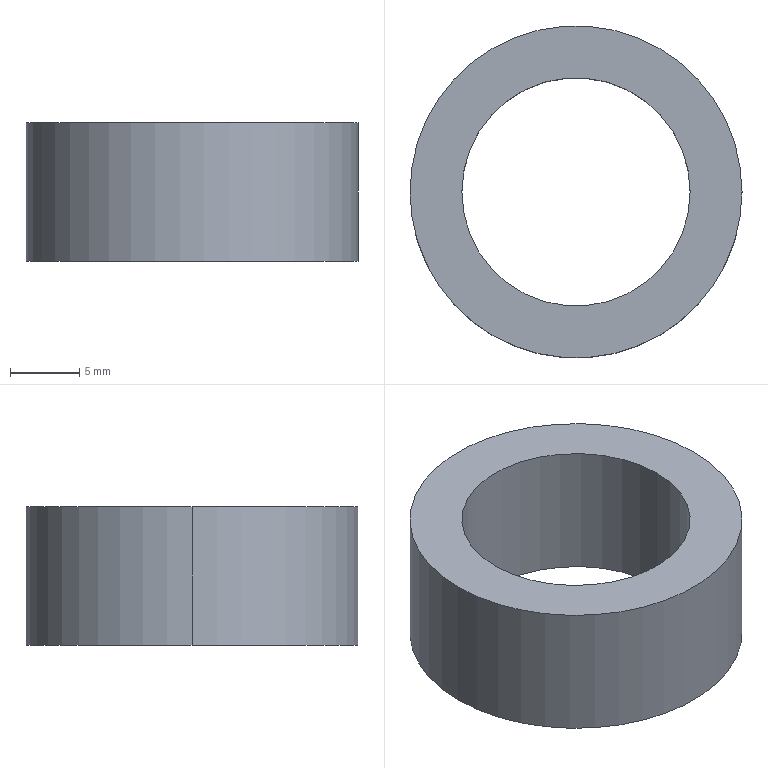Part | SolidWorks | features Extrusion 1 | 1 solid | 6 faces | box 24 x 24 x 10 mm | volume 2386 mm3 | cylinder 4 | plane 2 | commonest cylinder face diameters 16.5 x2 24 x2
STEP:
#1=CARTESIAN_POINT('',(-8.25,0.,10.));
#2=VERTEX_POINT('',#1);
#3=CARTESIAN_POINT('',(8.25,0.,10.));
#4=VERTEX_POINT('',#3);
#5=CARTESIAN_POINT('',(0.,0.,10.));
#6=DIRECTION('',(0.,0.,1.));
#7=DIRECTION('',(1.,0.,0.));
#8=AXIS2_PLACEMENT_3D('',#5,#6,#7);
#9=CIRCLE('',#8,8.25);
#10=EDGE_CURVE('',#2,#4,#9,.T.);
#11=ORIENTED_EDGE('',*,*,#10,.T.);
#12=CARTESIAN_POINT('',(8.25,0.,0.));
#13=VERTEX_POINT('',#12);
#14=CARTESIAN_POINT('',(8.25,0.,10.));
#15=DIRECTION('',(0.,0.,-1.));
#16=VECTOR('',#15,1000.);
#17=LINE('',#14,#16);
#18=EDGE_CURVE('',#4,#13,#17,.T.);
#19=ORIENTED_EDGE('',*,*,#18,.T.);
#20=CARTESIAN_POINT('',(-8.25,0.,0.));
#21=VERTEX_POINT('',#20);
#22=CARTESIAN_POINT('',(0.,0.,0.));
#23=DIRECTION('',(0.,0.,1.));
#24=DIRECTION('',(1.,0.,0.));
#25=AXIS2_PLACEMENT_3D('',#22,#23,#24);
#26=CIRCLE('',#25,8.25);
#27=EDGE_CURVE('',#21,#13,#26,.T.);
#28=ORIENTED_EDGE('',*,*,#27,.F.);
#29=CARTESIAN_POINT('',(-8.25,0.,10.));
#30=DIRECTION('',(0.,0.,-1.));
#31=VECTOR('',#30,1000.);
#32=LINE('',#29,#31);
#33=EDGE_CURVE('',#2,#21,#32,.T.);
#34=ORIENTED_EDGE('',*,*,#33,.F.);
#35=EDGE_LOOP('',(#11,#19,#28,#34));
#36=FACE_OUTER_BOUND('',#35,.T.);
#37=CARTESIAN_POINT('',(0.,0.,10.));
#38=DIRECTION('',(0.,0.,-1.));
#39=DIRECTION('',(-1.,0.,0.));
#40=AXIS2_PLACEMENT_3D('',#37,#38,#39);
#41=CYLINDRICAL_SURFACE('',#40,8.25);
#42=ADVANCED_FACE('',(#36),#41,.F.);
#43=CARTESIAN_POINT('',(12.,0.,10.));
#44=VERTEX_POINT('',#43);
#45=CARTESIAN_POINT('',(-12.,0.,10.));
#46=VERTEX_POINT('',#45);
#47=CARTESIAN_POINT('',(0.,0.,10.));
#48=DIRECTION('',(0.,0.,1.));
#49=DIRECTION('',(1.,0.,0.));
#50=AXIS2_PLACEMENT_3D('',#47,#48,#49);
#51=CIRCLE('',#50,12.);
#52=EDGE_CURVE('',#44,#46,#51,.T.);
#53=ORIENTED_EDGE('',*,*,#52,.F.);
#54=CARTESIAN_POINT('',(12.,0.,0.));
#55=VERTEX_POINT('',#54);
#56=CARTESIAN_POINT('',(12.,0.,10.));
#57=DIRECTION('',(0.,0.,-1.));
#58=VECTOR('',#57,1000.);
#59=LINE('',#56,#58);
#60=EDGE_CURVE('',#44,#55,#59,.T.);
#61=ORIENTED_EDGE('',*,*,#60,.T.);
#62=CARTESIAN_POINT('',(-12.,0.,0.));
#63=VERTEX_POINT('',#62);
#64=CARTESIAN_POINT('',(0.,0.,0.));
#65=DIRECTION('',(0.,0.,1.));
#66=DIRECTION('',(1.,0.,0.));
#67=AXIS2_PLACEMENT_3D('',#64,#65,#66);
#68=CIRCLE('',#67,12.);
#69=EDGE_CURVE('',#55,#63,#68,.T.);
#70=ORIENTED_EDGE('',*,*,#69,.T.);
#71=CARTESIAN_POINT('',(-12.,0.,10.));
#72=DIRECTION('',(0.,0.,-1.));
#73=VECTOR('',#72,1000.);
#74=LINE('',#71,#73);
#75=EDGE_CURVE('',#46,#63,#74,.T.);
#76=ORIENTED_EDGE('',*,*,#75,.F.);
#77=EDGE_LOOP('',(#53,#61,#70,#76));
#78=FACE_OUTER_BOUND('',#77,.T.);
#79=CARTESIAN_POINT('',(0.,0.,10.));
#80=DIRECTION('',(0.,0.,-1.));
#81=DIRECTION('',(-1.,0.,0.));
#82=AXIS2_PLACEMENT_3D('',#79,#80,#81);
#83=CYLINDRICAL_SURFACE('',#82,12.);
#84=ADVANCED_FACE('',(#78),#83,.T.);
#85=CARTESIAN_POINT('',(0.,0.,10.));
#86=DIRECTION('',(0.,0.,1.));
#87=DIRECTION('',(1.,0.,0.));
#88=AXIS2_PLACEMENT_3D('',#85,#86,#87);
#89=CIRCLE('',#88,12.);
#90=EDGE_CURVE('',#46,#44,#89,.T.);
#91=ORIENTED_EDGE('',*,*,#90,.T.);
#92=ORIENTED_EDGE('',*,*,#52,.T.);
#93=EDGE_LOOP('',(#91,#92));
#94=FACE_OUTER_BOUND('',#93,.T.);
#95=ORIENTED_EDGE('',*,*,#10,.F.);
#96=CARTESIAN_POINT('',(0.,0.,10.));
#97=DIRECTION('',(0.,0.,1.));
#98=DIRECTION('',(1.,0.,0.));
#99=AXIS2_PLACEMENT_3D('',#96,#97,#98);
#100=CIRCLE('',#99,8.25);
#101=EDGE_CURVE('',#4,#2,#100,.T.);
#102=ORIENTED_EDGE('',*,*,#101,.F.);
#103=EDGE_LOOP('',(#95,#102));
#104=FACE_BOUND('',#103,.T.);
#105=CARTESIAN_POINT('',(0.,0.,10.));
#106=DIRECTION('',(0.,0.,1.));
#107=DIRECTION('',(1.,0.,0.));
#108=AXIS2_PLACEMENT_3D('',#105,#106,#107);
#109=PLANE('',#108);
#110=ADVANCED_FACE('',(#94,#104),#109,.T.);
#111=CARTESIAN_POINT('',(0.,0.,0.));
#112=DIRECTION('',(0.,0.,1.));
#113=DIRECTION('',(1.,0.,0.));
#114=AXIS2_PLACEMENT_3D('',#111,#112,#113);
#115=CIRCLE('',#114,12.);
#116=EDGE_CURVE('',#63,#55,#115,.T.);
#117=ORIENTED_EDGE('',*,*,#116,.F.);
#118=ORIENTED_EDGE('',*,*,#69,.F.);
#119=EDGE_LOOP('',(#117,#118));
#120=FACE_OUTER_BOUND('',#119,.T.);
#121=ORIENTED_EDGE('',*,*,#27,.T.);
#122=CARTESIAN_POINT('',(0.,0.,0.));
#123=DIRECTION('',(0.,0.,1.));
#124=DIRECTION('',(1.,0.,0.));
#125=AXIS2_PLACEMENT_3D('',#122,#123,#124);
#126=CIRCLE('',#125,8.25);
#127=EDGE_CURVE('',#13,#21,#126,.T.);
#128=ORIENTED_EDGE('',*,*,#127,.T.);
#129=EDGE_LOOP('',(#121,#128));
#130=FACE_BOUND('',#129,.T.);
#131=CARTESIAN_POINT('',(0.,0.,0.));
#132=DIRECTION('',(0.,0.,1.));
#133=DIRECTION('',(1.,0.,0.));
#134=AXIS2_PLACEMENT_3D('',#131,#132,#133);
#135=PLANE('',#134);
#136=ADVANCED_FACE('',(#120,#130),#135,.F.);
#137=ORIENTED_EDGE('',*,*,#60,.F.);
#138=ORIENTED_EDGE('',*,*,#90,.F.);
#139=ORIENTED_EDGE('',*,*,#75,.T.);
#140=ORIENTED_EDGE('',*,*,#116,.T.);
#141=EDGE_LOOP('',(#137,#138,#139,#140));
#142=FACE_OUTER_BOUND('',#141,.T.);
#143=CARTESIAN_POINT('',(0.,0.,10.));
#144=DIRECTION('',(0.,0.,-1.));
#145=DIRECTION('',(-1.,0.,0.));
#146=AXIS2_PLACEMENT_3D('',#143,#144,#145);
#147=CYLINDRICAL_SURFACE('',#146,12.);
#148=ADVANCED_FACE('',(#142),#147,.T.);
#149=ORIENTED_EDGE('',*,*,#18,.F.);
#150=ORIENTED_EDGE('',*,*,#101,.T.);
#151=ORIENTED_EDGE('',*,*,#33,.T.);
#152=ORIENTED_EDGE('',*,*,#127,.F.);
#153=EDGE_LOOP('',(#149,#150,#151,#152));
#154=FACE_OUTER_BOUND('',#153,.T.);
#155=CARTESIAN_POINT('',(0.,0.,10.));
#156=DIRECTION('',(0.,0.,-1.));
#157=DIRECTION('',(-1.,0.,0.));
#158=AXIS2_PLACEMENT_3D('',#155,#156,#157);
#159=CYLINDRICAL_SURFACE('',#158,8.25);
#160=ADVANCED_FACE('',(#154),#159,.F.);
#161=CLOSED_SHELL('',(#42,#84,#110,#136,#148,#160));
#162=MANIFOLD_SOLID_BREP('',#161);
#163=CARTESIAN_POINT('',(0.,0.,0.));
#164=DIRECTION('',(0.,0.,1.));
#165=DIRECTION('',(1.,0.,0.));
#166=AXIS2_PLACEMENT_3D('',#163,#164,#165);
#167=(LENGTH_UNIT()NAMED_UNIT(*)SI_UNIT(.MILLI.,.METRE.));
#168=UNCERTAINTY_MEASURE_WITH_UNIT(LENGTH_MEASURE(0.00001),#167,'','');
#169=(NAMED_UNIT(*)PLANE_ANGLE_UNIT()SI_UNIT($,.RADIAN.));
#170=(NAMED_UNIT(*)SI_UNIT($,.STERADIAN.)SOLID_ANGLE_UNIT());
#171=(GEOMETRIC_REPRESENTATION_CONTEXT(3)GLOBAL_UNCERTAINTY_ASSIGNED_CONTEXT((#168))GLOBAL_UNIT_ASSIGNED_CONTEXT((#167,#169,#170))REPRESENTATION_CONTEXT('',''));
#172=ADVANCED_BREP_SHAPE_REPRESENTATION('',(#162,#166),#171);